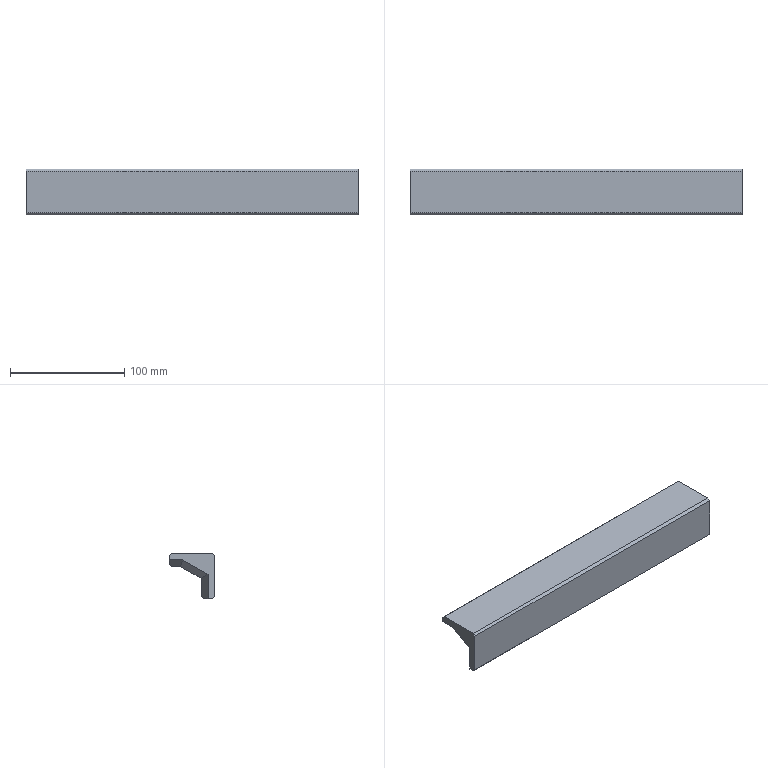CAM job | NX | 3+2 milling | part box 290 x 40 x 40 mm | stock box 295 x 45 x 45 mm
Tools:
number,name,description,diameter,corner_radius,flute_length,length,flutes
9,D10,平底铣刀-粗,10.0,0.0,35.0,75.0,2
10,D10-J,平底铣刀-精,10.0,0.0,35.0,75.0,2
17,D6R0.5,圆鼻刀-粗,6.0,0.5,50.0,75.0,2
1,D80R0.8FLYCUTTER,圆鼻刀-粗,80.0,0.8,50.0,75.0,2
1,D80R0.8FLYCUTTER-J,圆鼻刀-精,80.0,0.8,50.0,75.0,2
2,D6CHAMFER,倒角刀,6.0,0.0,3.0,25.0,2
Operations:
program,operation,operation_type,tool,method,geometry_group,spindle_rpm,surface_speed,feed_per_tooth,feed_cut,feed_plunge,cut_length_mm,path_length_mm,cut_time_min,machine_time_min
B,FLOORWALLFLYROUGH_COPY,VolumeBased25DMillingOperation,D80R0.8FLYCUTTER,LAYERROUGH-DEPTHK-STEPG,W-B,2800.0,703.696,0.5357,3000.0,100.0,3583.746,6935.966,1.195,1.53
B,FLOORWALLFLYFINISH_COPY,VolumeBased25DMillingOperation,D80R0.8FLYCUTTER-J,SIDEFINISH-DEPTHK-STEPG,W-B,4000.0,1005.28,0.125,1000.0,100.0,397.998,433.998,0.398,0.4016
B,CAVITYROUGH-MED_COPY,CavityMilling,D10,LAYERROUGH-DEPTHK-STEPG,W-B,8000.0,251.327,0.3125,5000.0,100.0,90734.746,92564.984,18.147,18.427
B,CAVITYROUGH-MED_COPY_COPY,CavityMilling,D10,LAYERROUGH-DEPTHK-STEPG,W-B,8000.0,251.32,0.25,4000.0,100.0,896.053,1202.102,0.224,0.2653
B,ZLEVELFINISHWALL_COPY_COPY,ZLevelMilling,D10,ZLEVELWALL-DEPTHK-STEPG,W-B,7000.0,219.911,0.3214,4500.0,100.0,4394.171,4424.812,0.9765,0.9795
B,FLOORWALLCHAMFER_COPY_1,VolumeBased25DMillingOperation,D6CHAMFER,WALLCHAMFER-DEPTH0-STEPG,W-B,6500.0,122.522,0.0769,1000.0,100.0,594.32,696.327,0.5943,0.6045
B,C0.3CLOSEDCONTOURCHAMFER6X45L_COPY,PlanarMilling,D6CHAMFER,WALLCHAMFER-DEPTH0-STEPG,W-B,7000.0,131.0,0.0714,1000.0,100.0,299.2,395.4,0.2992,0.3088
B,PLANEDEBURR6X45L_COPY,SurfaceContour,D6CHAMFER,WALLCHAMFER-DEPTH0-STEPG,W-B,6500.0,122.519,0.1154,1500.0,100.0,50.762,503.039,0.0338,0.0791
B,ZLEVELFINISH-MED_COPY,ZLevelMilling,D10-J,SIDEFINISH-DEPTHK-STEPG,W-B,8000.0,251.32,0.0625,1000.0,100.0,301.13,338.13,0.3011,0.3048
B,FLOORWALLFINISHBOTTOM-MED_COPY,VolumeBased25DMillingOperation,D10-J,FINISH-STEPDEPTHOFF,W-B,7000.0,175.0,0.0536,1500.0,100.0,1178.435,1260.435,0.7856,0.7938
B,FLOORWALLFINISHSIDE-MED-SELBOTTOM_COPY,VolumeBased25DMillingOperation,D10-J,SIDEFINISH-DEPTHK-STEPG,W-B,8000.0,251.32,0.0625,1000.0,100.0,295.623,378.623,0.2956,0.3039
B,ZLEVELFINISHWALL_COPY_COPY_COPY,ZLevelMilling,D6R0.5,ZLEVELWALL-DEPTHK-STEPG,W-B,7000.0,219.911,0.3214,4500.0,100.0,61022.63,61089.23,13.561,13.567
B,ZLEVELFINISHWALL_COPY_1,ZLevelMilling,D6R0.5,ZLEVELWALL-DEPTHK-STEPG,W-B,7000.0,131.947,0.2857,4000.0,100.0,3168.599,3259.624,0.7921,0.8013
A,TOPFACE,FaceMilling,D80R0.8FLYCUTTER,SIDEFINISH-DEPTHK-STEPG,W-A,4000.0,1005.31,0.125,1000.0,100.0,384.0,420.0,0.384,0.3876
A,PROFILE-ROUGH_2,VolumeBased25DMillingOperation,D10,METHOD,W-A,8000.0,251.327,0.3125,5000.0,80.0,36679.868,36758.868,7.336,7.344
A,ZLEVELFINISHWALL_COPY,ZLevelMilling,D10,ZLEVELWALL-DEPTHK-STEPG,W-A,7000.0,219.911,0.3214,4500.0,100.0,8788.341,8884.026,1.953,1.962
A,FLOORWALLCHAMFER_COPY,VolumeBased25DMillingOperation,D6CHAMFER,WALLCHAMFER-DEPTH0-STEPG,W-A,6500.0,122.522,0.0769,1000.0,100.0,603.03,730.862,0.603,0.6158
A,SOLIDONLY,SurfaceContour,D6CHAMFER,METHOD,W-A,8000.0,150.796,0.1875,3000.0,100.0,91.631,452.307,0.0305,0.0666
A,PROFILE-SEMIFINISH_2,VolumeBased25DMillingOperation,D10-J,METHOD,W-A,8000.0,251.327,0.0625,1000.0,100.0,2089.122,2373.151,2.089,2.118